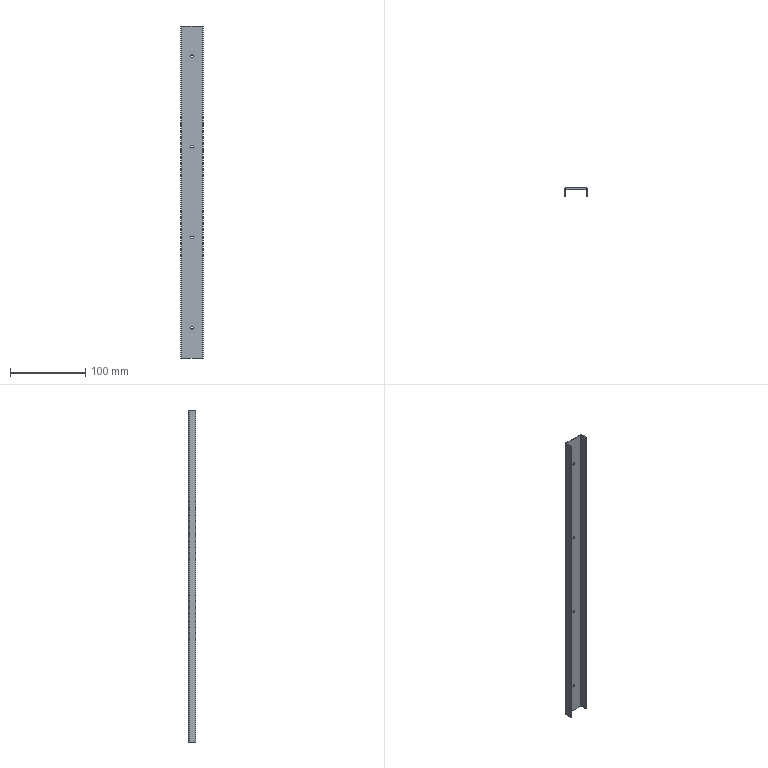Part | STEP file | 1 solid | 30 faces | box 30 x 10 x 440 mm | volume 30430 mm3 | plane 18 | cylinder 12 | commonest cylinder face diameters 3.3 x8 0.4 x2 3.4 x2